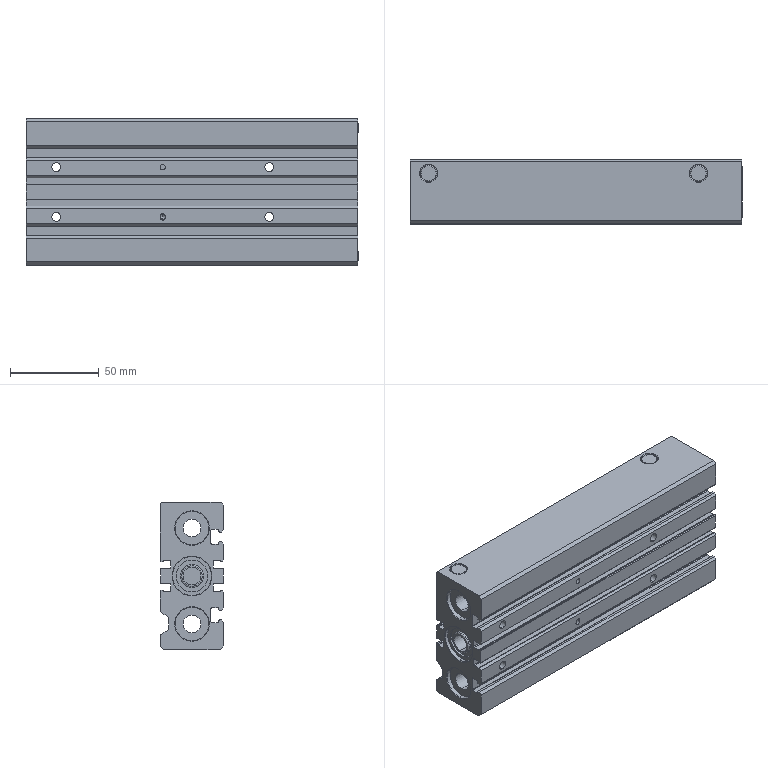Part | SolidWorks | features BaseBody 1 | 1 solid | 299 faces | box 187 x 36 x 83 mm | volume 380499 mm3 | cylinder 138 | plane 99 | cone 60 | spline 2 | commonest cylinder face diameters 0.8 x20 3 x14 0.4 x12 0.6 x10 10 x10 4.134 x8